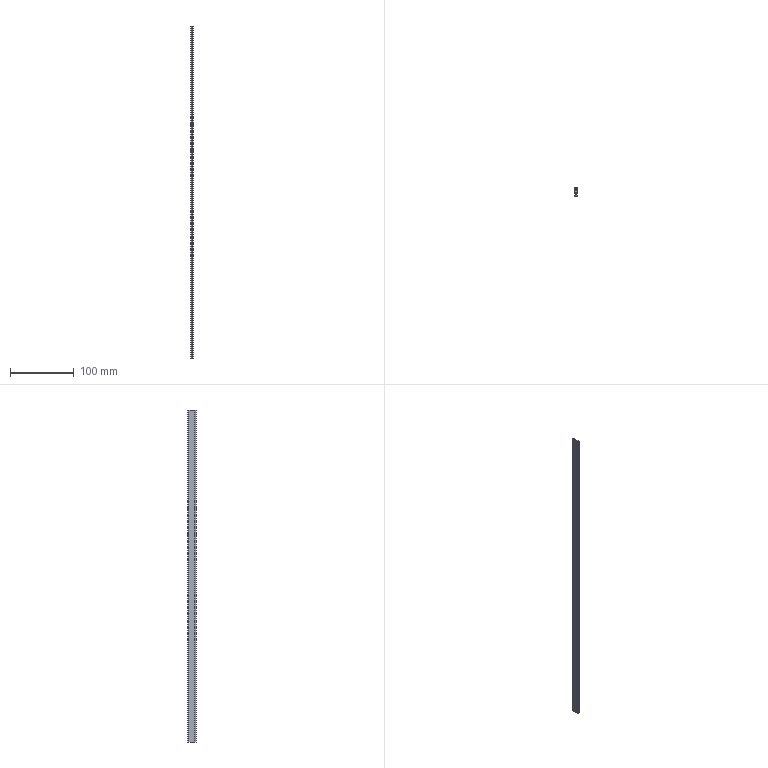Part | STEP file | 64685163 | 1 solid | 22 faces | box 4.361 x 13.946 x 520 mm | volume 14891 mm3 | plane 12 | cylinder 10 | commonest cylinder face diameters 0.48 x4 1 x2 3 x2 2 x1 4 x1